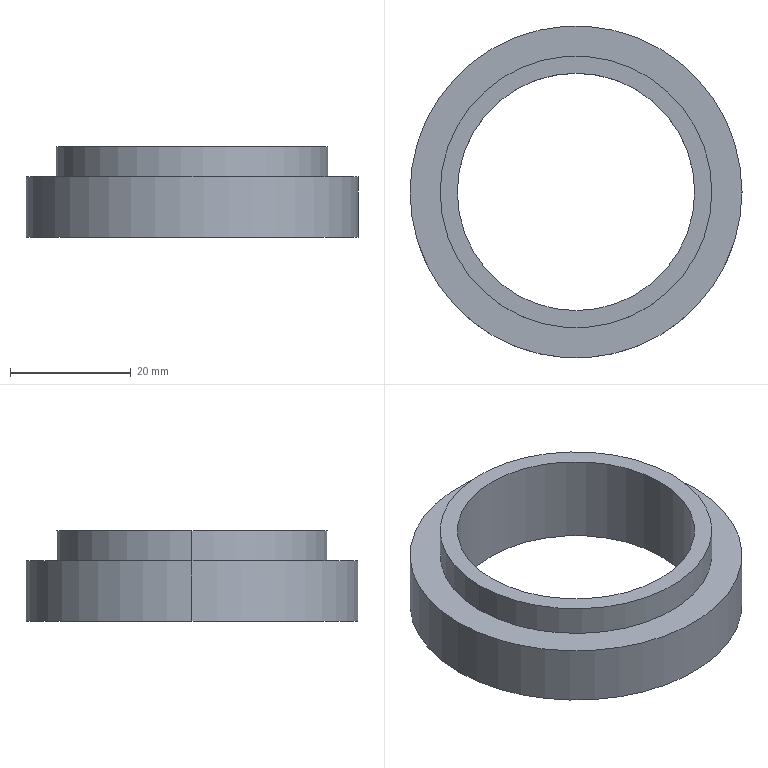Part | SolidWorks | features Extrusion 1, ICE 1 | 1 solid | 9 faces | box 55 x 55 x 15 mm | volume 13492 mm3 | cylinder 6 | plane 3 | commonest cylinder face diameters 39.325 x2 45 x2 55 x2
STEP:
#1=CARTESIAN_POINT('',(22.5,0.,15.));
#2=VERTEX_POINT('',#1);
#3=CARTESIAN_POINT('',(-22.5,0.,15.));
#4=VERTEX_POINT('',#3);
#5=CARTESIAN_POINT('',(0.,0.,15.));
#6=DIRECTION('',(0.,0.,1.));
#7=DIRECTION('',(1.,0.,0.));
#8=AXIS2_PLACEMENT_3D('',#5,#6,#7);
#9=CIRCLE('',#8,22.5);
#10=EDGE_CURVE('',#2,#4,#9,.T.);
#11=ORIENTED_EDGE('',*,*,#10,.F.);
#12=CARTESIAN_POINT('',(22.5,0.,10.));
#13=VERTEX_POINT('',#12);
#14=CARTESIAN_POINT('',(22.5,0.,15.));
#15=DIRECTION('',(0.,0.,-1.));
#16=VECTOR('',#15,1000.);
#17=LINE('',#14,#16);
#18=EDGE_CURVE('',#2,#13,#17,.T.);
#19=ORIENTED_EDGE('',*,*,#18,.T.);
#20=CARTESIAN_POINT('',(-22.5,0.,10.));
#21=VERTEX_POINT('',#20);
#22=CARTESIAN_POINT('',(0.,0.,10.));
#23=DIRECTION('',(0.,0.,1.));
#24=DIRECTION('',(1.,0.,0.));
#25=AXIS2_PLACEMENT_3D('',#22,#23,#24);
#26=CIRCLE('',#25,22.5);
#27=EDGE_CURVE('',#13,#21,#26,.T.);
#28=ORIENTED_EDGE('',*,*,#27,.T.);
#29=CARTESIAN_POINT('',(-22.5,0.,15.));
#30=DIRECTION('',(0.,0.,-1.));
#31=VECTOR('',#30,1000.);
#32=LINE('',#29,#31);
#33=EDGE_CURVE('',#4,#21,#32,.T.);
#34=ORIENTED_EDGE('',*,*,#33,.F.);
#35=EDGE_LOOP('',(#11,#19,#28,#34));
#36=FACE_OUTER_BOUND('',#35,.T.);
#37=CARTESIAN_POINT('',(0.,0.,15.));
#38=DIRECTION('',(0.,0.,-1.));
#39=DIRECTION('',(-1.,0.,0.));
#40=AXIS2_PLACEMENT_3D('',#37,#38,#39);
#41=CYLINDRICAL_SURFACE('',#40,22.5);
#42=ADVANCED_FACE('',(#36),#41,.T.);
#43=CARTESIAN_POINT('',(-19.662,0.,15.));
#44=VERTEX_POINT('',#43);
#45=CARTESIAN_POINT('',(19.662,0.,15.));
#46=VERTEX_POINT('',#45);
#47=CARTESIAN_POINT('',(0.,0.,15.));
#48=DIRECTION('',(0.,0.,1.));
#49=DIRECTION('',(1.,0.,0.));
#50=AXIS2_PLACEMENT_3D('',#47,#48,#49);
#51=CIRCLE('',#50,19.662);
#52=EDGE_CURVE('',#44,#46,#51,.T.);
#53=ORIENTED_EDGE('',*,*,#52,.T.);
#54=CARTESIAN_POINT('',(19.662,0.,0.));
#55=VERTEX_POINT('',#54);
#56=CARTESIAN_POINT('',(19.662,0.,10.));
#57=DIRECTION('',(0.,0.,-1.));
#58=VECTOR('',#57,1000.);
#59=LINE('',#56,#58);
#60=EDGE_CURVE('',#46,#55,#59,.T.);
#61=ORIENTED_EDGE('',*,*,#60,.T.);
#62=CARTESIAN_POINT('',(-19.662,0.,0.));
#63=VERTEX_POINT('',#62);
#64=CARTESIAN_POINT('',(0.,0.,0.));
#65=DIRECTION('',(0.,0.,1.));
#66=DIRECTION('',(1.,0.,0.));
#67=AXIS2_PLACEMENT_3D('',#64,#65,#66);
#68=CIRCLE('',#67,19.662);
#69=EDGE_CURVE('',#63,#55,#68,.T.);
#70=ORIENTED_EDGE('',*,*,#69,.F.);
#71=CARTESIAN_POINT('',(-19.662,0.,10.));
#72=DIRECTION('',(0.,0.,-1.));
#73=VECTOR('',#72,1000.);
#74=LINE('',#71,#73);
#75=EDGE_CURVE('',#44,#63,#74,.T.);
#76=ORIENTED_EDGE('',*,*,#75,.F.);
#77=EDGE_LOOP('',(#53,#61,#70,#76));
#78=FACE_OUTER_BOUND('',#77,.T.);
#79=CARTESIAN_POINT('',(0.,0.,10.));
#80=DIRECTION('',(0.,0.,-1.));
#81=DIRECTION('',(-1.,0.,0.));
#82=AXIS2_PLACEMENT_3D('',#79,#80,#81);
#83=CYLINDRICAL_SURFACE('',#82,19.662);
#84=ADVANCED_FACE('',(#78),#83,.F.);
#85=CARTESIAN_POINT('',(27.5,0.,10.));
#86=VERTEX_POINT('',#85);
#87=CARTESIAN_POINT('',(-27.5,0.,10.));
#88=VERTEX_POINT('',#87);
#89=CARTESIAN_POINT('',(0.,0.,10.));
#90=DIRECTION('',(0.,0.,1.));
#91=DIRECTION('',(1.,0.,0.));
#92=AXIS2_PLACEMENT_3D('',#89,#90,#91);
#93=CIRCLE('',#92,27.5);
#94=EDGE_CURVE('',#86,#88,#93,.T.);
#95=ORIENTED_EDGE('',*,*,#94,.F.);
#96=CARTESIAN_POINT('',(27.5,0.,0.));
#97=VERTEX_POINT('',#96);
#98=CARTESIAN_POINT('',(27.5,0.,10.));
#99=DIRECTION('',(0.,0.,-1.));
#100=VECTOR('',#99,1000.);
#101=LINE('',#98,#100);
#102=EDGE_CURVE('',#86,#97,#101,.T.);
#103=ORIENTED_EDGE('',*,*,#102,.T.);
#104=CARTESIAN_POINT('',(-27.5,0.,0.));
#105=VERTEX_POINT('',#104);
#106=CARTESIAN_POINT('',(0.,0.,0.));
#107=DIRECTION('',(0.,0.,1.));
#108=DIRECTION('',(1.,0.,0.));
#109=AXIS2_PLACEMENT_3D('',#106,#107,#108);
#110=CIRCLE('',#109,27.5);
#111=EDGE_CURVE('',#97,#105,#110,.T.);
#112=ORIENTED_EDGE('',*,*,#111,.T.);
#113=CARTESIAN_POINT('',(-27.5,0.,10.));
#114=DIRECTION('',(0.,0.,-1.));
#115=VECTOR('',#114,1000.);
#116=LINE('',#113,#115);
#117=EDGE_CURVE('',#88,#105,#116,.T.);
#118=ORIENTED_EDGE('',*,*,#117,.F.);
#119=EDGE_LOOP('',(#95,#103,#112,#118));
#120=FACE_OUTER_BOUND('',#119,.T.);
#121=CARTESIAN_POINT('',(0.,0.,10.));
#122=DIRECTION('',(0.,0.,-1.));
#123=DIRECTION('',(-1.,0.,0.));
#124=AXIS2_PLACEMENT_3D('',#121,#122,#123);
#125=CYLINDRICAL_SURFACE('',#124,27.5);
#126=ADVANCED_FACE('',(#120),#125,.T.);
#127=CARTESIAN_POINT('',(0.,0.,10.));
#128=DIRECTION('',(0.,0.,1.));
#129=DIRECTION('',(1.,0.,0.));
#130=AXIS2_PLACEMENT_3D('',#127,#128,#129);
#131=CIRCLE('',#130,27.5);
#132=EDGE_CURVE('',#88,#86,#131,.T.);
#133=ORIENTED_EDGE('',*,*,#132,.T.);
#134=ORIENTED_EDGE('',*,*,#94,.T.);
#135=EDGE_LOOP('',(#133,#134));
#136=FACE_OUTER_BOUND('',#135,.T.);
#137=CARTESIAN_POINT('',(0.,0.,10.));
#138=DIRECTION('',(0.,0.,1.));
#139=DIRECTION('',(1.,0.,0.));
#140=AXIS2_PLACEMENT_3D('',#137,#138,#139);
#141=CIRCLE('',#140,22.5);
#142=EDGE_CURVE('',#21,#13,#141,.T.);
#143=ORIENTED_EDGE('',*,*,#142,.F.);
#144=ORIENTED_EDGE('',*,*,#27,.F.);
#145=EDGE_LOOP('',(#143,#144));
#146=FACE_BOUND('',#145,.T.);
#147=CARTESIAN_POINT('',(0.,0.,10.));
#148=DIRECTION('',(0.,0.,1.));
#149=DIRECTION('',(1.,0.,0.));
#150=AXIS2_PLACEMENT_3D('',#147,#148,#149);
#151=PLANE('',#150);
#152=ADVANCED_FACE('',(#136,#146),#151,.T.);
#153=CARTESIAN_POINT('',(0.,0.,0.));
#154=DIRECTION('',(0.,0.,1.));
#155=DIRECTION('',(1.,0.,0.));
#156=AXIS2_PLACEMENT_3D('',#153,#154,#155);
#157=CIRCLE('',#156,27.5);
#158=EDGE_CURVE('',#105,#97,#157,.T.);
#159=ORIENTED_EDGE('',*,*,#158,.F.);
#160=ORIENTED_EDGE('',*,*,#111,.F.);
#161=EDGE_LOOP('',(#159,#160));
#162=FACE_OUTER_BOUND('',#161,.T.);
#163=ORIENTED_EDGE('',*,*,#69,.T.);
#164=CARTESIAN_POINT('',(0.,0.,0.));
#165=DIRECTION('',(0.,0.,1.));
#166=DIRECTION('',(1.,0.,0.));
#167=AXIS2_PLACEMENT_3D('',#164,#165,#166);
#168=CIRCLE('',#167,19.662);
#169=EDGE_CURVE('',#55,#63,#168,.T.);
#170=ORIENTED_EDGE('',*,*,#169,.T.);
#171=EDGE_LOOP('',(#163,#170));
#172=FACE_BOUND('',#171,.T.);
#173=CARTESIAN_POINT('',(0.,0.,0.));
#174=DIRECTION('',(0.,0.,1.));
#175=DIRECTION('',(1.,0.,0.));
#176=AXIS2_PLACEMENT_3D('',#173,#174,#175);
#177=PLANE('',#176);
#178=ADVANCED_FACE('',(#162,#172),#177,.F.);
#179=ORIENTED_EDGE('',*,*,#102,.F.);
#180=ORIENTED_EDGE('',*,*,#132,.F.);
#181=ORIENTED_EDGE('',*,*,#117,.T.);
#182=ORIENTED_EDGE('',*,*,#158,.T.);
#183=EDGE_LOOP('',(#179,#180,#181,#182));
#184=FACE_OUTER_BOUND('',#183,.T.);
#185=CARTESIAN_POINT('',(0.,0.,10.));
#186=DIRECTION('',(0.,0.,-1.));
#187=DIRECTION('',(-1.,0.,0.));
#188=AXIS2_PLACEMENT_3D('',#185,#186,#187);
#189=CYLINDRICAL_SURFACE('',#188,27.5);
#190=ADVANCED_FACE('',(#184),#189,.T.);
#191=ORIENTED_EDGE('',*,*,#60,.F.);
#192=CARTESIAN_POINT('',(0.,0.,15.));
#193=DIRECTION('',(0.,0.,1.));
#194=DIRECTION('',(1.,0.,0.));
#195=AXIS2_PLACEMENT_3D('',#192,#193,#194);
#196=CIRCLE('',#195,19.662);
#197=EDGE_CURVE('',#46,#44,#196,.T.);
#198=ORIENTED_EDGE('',*,*,#197,.T.);
#199=ORIENTED_EDGE('',*,*,#75,.T.);
#200=ORIENTED_EDGE('',*,*,#169,.F.);
#201=EDGE_LOOP('',(#191,#198,#199,#200));
#202=FACE_OUTER_BOUND('',#201,.T.);
#203=CARTESIAN_POINT('',(0.,0.,10.));
#204=DIRECTION('',(0.,0.,-1.));
#205=DIRECTION('',(-1.,0.,0.));
#206=AXIS2_PLACEMENT_3D('',#203,#204,#205);
#207=CYLINDRICAL_SURFACE('',#206,19.662);
#208=ADVANCED_FACE('',(#202),#207,.F.);
#209=CARTESIAN_POINT('',(0.,0.,15.));
#210=DIRECTION('',(0.,0.,1.));
#211=DIRECTION('',(1.,0.,0.));
#212=AXIS2_PLACEMENT_3D('',#209,#210,#211);
#213=CIRCLE('',#212,22.5);
#214=EDGE_CURVE('',#4,#2,#213,.T.);
#215=ORIENTED_EDGE('',*,*,#214,.T.);
#216=ORIENTED_EDGE('',*,*,#10,.T.);
#217=EDGE_LOOP('',(#215,#216));
#218=FACE_OUTER_BOUND('',#217,.T.);
#219=ORIENTED_EDGE('',*,*,#52,.F.);
#220=ORIENTED_EDGE('',*,*,#197,.F.);
#221=EDGE_LOOP('',(#219,#220));
#222=FACE_BOUND('',#221,.T.);
#223=CARTESIAN_POINT('',(0.,0.,15.));
#224=DIRECTION('',(0.,0.,1.));
#225=DIRECTION('',(1.,0.,0.));
#226=AXIS2_PLACEMENT_3D('',#223,#224,#225);
#227=PLANE('',#226);
#228=ADVANCED_FACE('',(#218,#222),#227,.T.);
#229=ORIENTED_EDGE('',*,*,#18,.F.);
#230=ORIENTED_EDGE('',*,*,#214,.F.);
#231=ORIENTED_EDGE('',*,*,#33,.T.);
#232=ORIENTED_EDGE('',*,*,#142,.T.);
#233=EDGE_LOOP('',(#229,#230,#231,#232));
#234=FACE_OUTER_BOUND('',#233,.T.);
#235=CARTESIAN_POINT('',(0.,0.,15.));
#236=DIRECTION('',(0.,0.,-1.));
#237=DIRECTION('',(-1.,0.,0.));
#238=AXIS2_PLACEMENT_3D('',#235,#236,#237);
#239=CYLINDRICAL_SURFACE('',#238,22.5);
#240=ADVANCED_FACE('',(#234),#239,.T.);
#241=CLOSED_SHELL('',(#42,#84,#126,#152,#178,#190,#208,#228,#240));
#242=MANIFOLD_SOLID_BREP('',#241);
#243=CARTESIAN_POINT('',(0.,0.,0.));
#244=DIRECTION('',(0.,0.,1.));
#245=DIRECTION('',(1.,0.,0.));
#246=AXIS2_PLACEMENT_3D('',#243,#244,#245);
#247=(LENGTH_UNIT()NAMED_UNIT(*)SI_UNIT(.MILLI.,.METRE.));
#248=UNCERTAINTY_MEASURE_WITH_UNIT(LENGTH_MEASURE(0.00001),#247,'','');
#249=(NAMED_UNIT(*)PLANE_ANGLE_UNIT()SI_UNIT($,.RADIAN.));
#250=(NAMED_UNIT(*)SI_UNIT($,.STERADIAN.)SOLID_ANGLE_UNIT());
#251=(GEOMETRIC_REPRESENTATION_CONTEXT(3)GLOBAL_UNCERTAINTY_ASSIGNED_CONTEXT((#248))GLOBAL_UNIT_ASSIGNED_CONTEXT((#247,#249,#250))REPRESENTATION_CONTEXT('',''));
#252=ADVANCED_BREP_SHAPE_REPRESENTATION('',(#242,#246),#251);